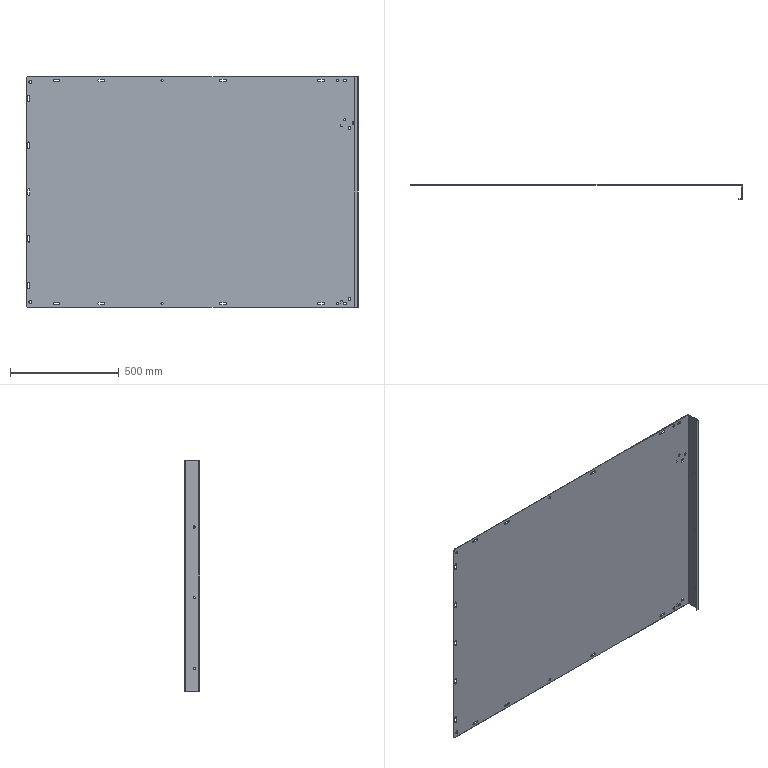Part | SolidWorks | features ICE 10, Cut 1, Fillet 1, FlatPattern 1, SMBaseFlange 1, SheetMetal 1 | 1 solid | 131 faces | box 1525 x 70 x 1060 mm | volume 5080133 mm3 | plane 68 | cylinder 63 | commonest cylinder face diameters 10 x39 10.5 x10 11 x4 12.8 x4 0.4 x2 6.4 x2